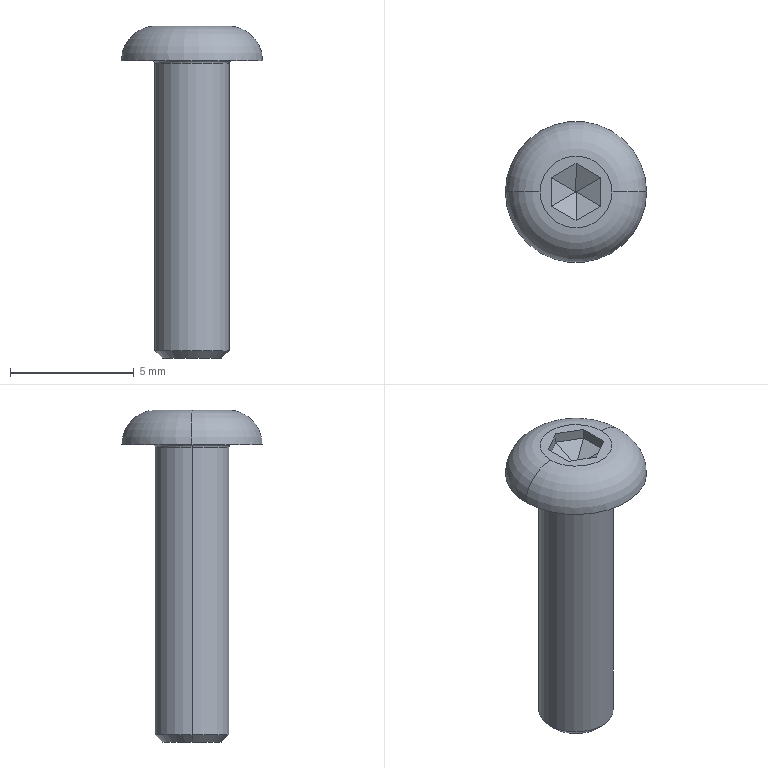Part | SolidWorks | features BaseBody 1 | 1 solid | 24 faces | box 5.7 x 5.7 x 13.4 mm | volume 111.333 mm3 | plane 16 | torus 4 | cone 2 | cylinder 2 | commonest cylinder face diameters 3 x2
STEP:
#1=CARTESIAN_POINT('',(-1.6,0.,0.));
#2=VERTEX_POINT('',#1);
#3=CARTESIAN_POINT('',(1.6,0.,0.));
#4=VERTEX_POINT('',#3);
#5=CARTESIAN_POINT('',(0.,0.,0.));
#6=DIRECTION('',(0.,0.,1.));
#7=DIRECTION('',(1.,0.,0.));
#8=AXIS2_PLACEMENT_3D('',#5,#6,#7);
#9=CIRCLE('',#8,1.6);
#10=EDGE_CURVE('',#2,#4,#9,.T.);
#11=ORIENTED_EDGE('',*,*,#10,.F.);
#12=CARTESIAN_POINT('',(-1.5,0.,-0.1));
#13=VERTEX_POINT('',#12);
#14=CARTESIAN_POINT('',(-1.6,0.,-0.1));
#15=DIRECTION('',(0.,1.,0.));
#16=DIRECTION('',(-1.,0.,0.));
#17=AXIS2_PLACEMENT_3D('',#14,#15,#16);
#18=CIRCLE('',#17,0.1);
#19=EDGE_CURVE('',#2,#13,#18,.T.);
#20=ORIENTED_EDGE('',*,*,#19,.T.);
#21=CARTESIAN_POINT('',(1.5,0.,-0.1));
#22=VERTEX_POINT('',#21);
#23=CARTESIAN_POINT('',(0.,0.,-0.1));
#24=DIRECTION('',(0.,0.,-1.));
#25=DIRECTION('',(1.,0.,0.));
#26=AXIS2_PLACEMENT_3D('',#23,#24,#25);
#27=CIRCLE('',#26,1.5);
#28=EDGE_CURVE('',#22,#13,#27,.T.);
#29=ORIENTED_EDGE('',*,*,#28,.F.);
#30=CARTESIAN_POINT('',(1.6,0.,-0.1));
#31=DIRECTION('',(0.,-1.,0.));
#32=DIRECTION('',(0.,0.,-1.));
#33=AXIS2_PLACEMENT_3D('',#30,#31,#32);
#34=CIRCLE('',#33,0.1);
#35=EDGE_CURVE('',#4,#22,#34,.T.);
#36=ORIENTED_EDGE('',*,*,#35,.F.);
#37=EDGE_LOOP('',(#11,#20,#29,#36));
#38=FACE_OUTER_BOUND('',#37,.T.);
#39=CARTESIAN_POINT('',(0.,0.,-0.1));
#40=DIRECTION('',(0.,0.,1.));
#41=DIRECTION('',(1.,0.,0.));
#42=AXIS2_PLACEMENT_3D('',#39,#40,#41);
#43=TOROIDAL_SURFACE('',#42,1.6,0.1);
#44=ADVANCED_FACE('',(#38),#43,.F.);
#45=CARTESIAN_POINT('',(-1.2,0.,-12.));
#46=VERTEX_POINT('',#45);
#47=CARTESIAN_POINT('',(1.2,0.,-12.));
#48=VERTEX_POINT('',#47);
#49=CARTESIAN_POINT('',(0.,0.,-12.));
#50=DIRECTION('',(0.,0.,-1.));
#51=DIRECTION('',(-1.,0.,0.));
#52=AXIS2_PLACEMENT_3D('',#49,#50,#51);
#53=CIRCLE('',#52,1.2);
#54=EDGE_CURVE('',#46,#48,#53,.T.);
#55=ORIENTED_EDGE('',*,*,#54,.F.);
#56=CARTESIAN_POINT('',(-1.5,0.,-11.7));
#57=VERTEX_POINT('',#56);
#58=CARTESIAN_POINT('',(-1.2,0.,-12.));
#59=DIRECTION('',(-0.7071,0.,0.7071));
#60=VECTOR('',#59,1000.);
#61=LINE('',#58,#60);
#62=EDGE_CURVE('',#46,#57,#61,.T.);
#63=ORIENTED_EDGE('',*,*,#62,.T.);
#64=CARTESIAN_POINT('',(1.5,0.,-11.7));
#65=VERTEX_POINT('',#64);
#66=CARTESIAN_POINT('',(0.,0.,-11.7));
#67=DIRECTION('',(0.,0.,1.));
#68=DIRECTION('',(-1.,0.,0.));
#69=AXIS2_PLACEMENT_3D('',#66,#67,#68);
#70=CIRCLE('',#69,1.5);
#71=EDGE_CURVE('',#65,#57,#70,.T.);
#72=ORIENTED_EDGE('',*,*,#71,.F.);
#73=CARTESIAN_POINT('',(1.2,0.,-12.));
#74=DIRECTION('',(0.7071,0.,0.7071));
#75=VECTOR('',#74,1000.);
#76=LINE('',#73,#75);
#77=EDGE_CURVE('',#48,#65,#76,.T.);
#78=ORIENTED_EDGE('',*,*,#77,.F.);
#79=EDGE_LOOP('',(#55,#63,#72,#78));
#80=FACE_OUTER_BOUND('',#79,.T.);
#81=CARTESIAN_POINT('',(0.,0.,-12.));
#82=DIRECTION('',(0.,0.,1.));
#83=DIRECTION('',(1.,0.,0.));
#84=AXIS2_PLACEMENT_3D('',#81,#82,#83);
#85=CONICAL_SURFACE('',#84,1.2,0.7854);
#86=ADVANCED_FACE('',(#80),#85,.T.);
#87=ORIENTED_EDGE('',*,*,#71,.T.);
#88=CARTESIAN_POINT('',(-1.5,0.,-12.));
#89=DIRECTION('',(0.,0.,1.));
#90=VECTOR('',#89,1000.);
#91=LINE('',#88,#90);
#92=EDGE_CURVE('',#57,#13,#91,.T.);
#93=ORIENTED_EDGE('',*,*,#92,.T.);
#94=CARTESIAN_POINT('',(0.,0.,-0.1));
#95=DIRECTION('',(0.,0.,-1.));
#96=DIRECTION('',(1.,0.,0.));
#97=AXIS2_PLACEMENT_3D('',#94,#95,#96);
#98=CIRCLE('',#97,1.5);
#99=EDGE_CURVE('',#13,#22,#98,.T.);
#100=ORIENTED_EDGE('',*,*,#99,.T.);
#101=CARTESIAN_POINT('',(1.5,0.,-12.));
#102=DIRECTION('',(0.,0.,1.));
#103=VECTOR('',#102,1000.);
#104=LINE('',#101,#103);
#105=EDGE_CURVE('',#65,#22,#104,.T.);
#106=ORIENTED_EDGE('',*,*,#105,.F.);
#107=EDGE_LOOP('',(#87,#93,#100,#106));
#108=FACE_OUTER_BOUND('',#107,.T.);
#109=CARTESIAN_POINT('',(0.,0.,-12.));
#110=DIRECTION('',(0.,0.,1.));
#111=DIRECTION('',(1.,0.,0.));
#112=AXIS2_PLACEMENT_3D('',#109,#110,#111);
#113=CYLINDRICAL_SURFACE('',#112,1.5);
#114=ADVANCED_FACE('',(#108),#113,.T.);
#115=CARTESIAN_POINT('',(2.85,0.,0.));
#116=VERTEX_POINT('',#115);
#117=CARTESIAN_POINT('',(-2.85,0.,0.));
#118=VERTEX_POINT('',#117);
#119=CARTESIAN_POINT('',(0.,0.,0.));
#120=DIRECTION('',(0.,0.,1.));
#121=DIRECTION('',(1.,0.,0.));
#122=AXIS2_PLACEMENT_3D('',#119,#120,#121);
#123=CIRCLE('',#122,2.85);
#124=EDGE_CURVE('',#116,#118,#123,.T.);
#125=ORIENTED_EDGE('',*,*,#124,.T.);
#126=CARTESIAN_POINT('',(-1.45,0.,1.4));
#127=VERTEX_POINT('',#126);
#128=CARTESIAN_POINT('',(-1.45,0.,0.));
#129=DIRECTION('',(0.,1.,0.));
#130=DIRECTION('',(-1.,0.,0.));
#131=AXIS2_PLACEMENT_3D('',#128,#129,#130);
#132=CIRCLE('',#131,1.4);
#133=EDGE_CURVE('',#118,#127,#132,.T.);
#134=ORIENTED_EDGE('',*,*,#133,.T.);
#135=CARTESIAN_POINT('',(1.45,0.,1.4));
#136=VERTEX_POINT('',#135);
#137=CARTESIAN_POINT('',(0.,0.,1.4));
#138=DIRECTION('',(0.,0.,1.));
#139=DIRECTION('',(1.,0.,0.));
#140=AXIS2_PLACEMENT_3D('',#137,#138,#139);
#141=CIRCLE('',#140,1.45);
#142=EDGE_CURVE('',#136,#127,#141,.T.);
#143=ORIENTED_EDGE('',*,*,#142,.F.);
#144=CARTESIAN_POINT('',(1.45,0.,0.));
#145=DIRECTION('',(0.,-1.,0.));
#146=DIRECTION('',(0.,0.,-1.));
#147=AXIS2_PLACEMENT_3D('',#144,#145,#146);
#148=CIRCLE('',#147,1.4);
#149=EDGE_CURVE('',#116,#136,#148,.T.);
#150=ORIENTED_EDGE('',*,*,#149,.F.);
#151=EDGE_LOOP('',(#125,#134,#143,#150));
#152=FACE_OUTER_BOUND('',#151,.T.);
#153=CARTESIAN_POINT('',(0.,0.,0.));
#154=DIRECTION('',(0.,0.,1.));
#155=DIRECTION('',(1.,0.,0.));
#156=AXIS2_PLACEMENT_3D('',#153,#154,#155);
#157=TOROIDAL_SURFACE('',#156,1.45,1.4);
#158=ADVANCED_FACE('',(#152),#157,.T.);
#159=CARTESIAN_POINT('',(-0.0017,-0.0009814,0.4));
#160=VERTEX_POINT('',#159);
#161=CARTESIAN_POINT('',(-1.,-0.5774,0.9764));
#162=VERTEX_POINT('',#161);
#163=CARTESIAN_POINT('',(-0.00136,-0.0007851,0.3998));
#164=DIRECTION('',(-0.7746,-0.4472,0.4472));
#165=VECTOR('',#164,1000.);
#166=LINE('',#163,#165);
#167=EDGE_CURVE('',#160,#162,#166,.T.);
#168=ORIENTED_EDGE('',*,*,#167,.T.);
#169=CARTESIAN_POINT('',(0.,-1.155,0.9764));
#170=VERTEX_POINT('',#169);
#171=CARTESIAN_POINT('',(-1.,-0.5774,0.9764));
#172=DIRECTION('',(-0.866,0.5,0.));
#173=VECTOR('',#172,1000.);
#174=LINE('',#171,#173);
#175=EDGE_CURVE('',#170,#162,#174,.T.);
#176=ORIENTED_EDGE('',*,*,#175,.F.);
#177=CARTESIAN_POINT('',(0.,-0.001963,0.4));
#178=VERTEX_POINT('',#177);
#179=CARTESIAN_POINT('',(0.,-0.00157,0.3998));
#180=DIRECTION('',(0.,0.8944,-0.4472));
#181=VECTOR('',#180,1000.);
#182=LINE('',#179,#181);
#183=EDGE_CURVE('',#170,#178,#182,.T.);
#184=ORIENTED_EDGE('',*,*,#183,.T.);
#185=CARTESIAN_POINT('',(-0.0008499,-0.001472,0.4));
#186=DIRECTION('',(0.866,-0.5,0.));
#187=VECTOR('',#186,1000.);
#188=LINE('',#185,#187);
#189=EDGE_CURVE('',#160,#178,#188,.T.);
#190=ORIENTED_EDGE('',*,*,#189,.F.);
#191=EDGE_LOOP('',(#168,#176,#184,#190));
#192=FACE_OUTER_BOUND('',#191,.T.);
#193=CARTESIAN_POINT('',(-0.0008499,-0.001472,0.4));
#194=DIRECTION('',(-0.25,-0.433,-0.866));
#195=DIRECTION('',(0.,-0.8944,0.4472));
#196=AXIS2_PLACEMENT_3D('',#193,#194,#195);
#197=PLANE('',#196);
#198=ADVANCED_FACE('',(#192),#197,.F.);
#199=CARTESIAN_POINT('',(1.,-0.5774,0.9764));
#200=VERTEX_POINT('',#199);
#201=CARTESIAN_POINT('',(0.0017,-0.0009814,0.4));
#202=VERTEX_POINT('',#201);
#203=CARTESIAN_POINT('',(0.00136,-0.0007851,0.3998));
#204=DIRECTION('',(-0.7746,0.4472,-0.4472));
#205=VECTOR('',#204,1000.);
#206=LINE('',#203,#205);
#207=EDGE_CURVE('',#200,#202,#206,.T.);
#208=ORIENTED_EDGE('',*,*,#207,.T.);
#209=CARTESIAN_POINT('',(0.0008499,-0.001472,0.4));
#210=DIRECTION('',(0.866,0.5,0.));
#211=VECTOR('',#210,1000.);
#212=LINE('',#209,#211);
#213=EDGE_CURVE('',#178,#202,#212,.T.);
#214=ORIENTED_EDGE('',*,*,#213,.F.);
#215=ORIENTED_EDGE('',*,*,#183,.F.);
#216=CARTESIAN_POINT('',(0.,-1.155,0.9764));
#217=DIRECTION('',(-0.866,-0.5,0.));
#218=VECTOR('',#217,1000.);
#219=LINE('',#216,#218);
#220=EDGE_CURVE('',#200,#170,#219,.T.);
#221=ORIENTED_EDGE('',*,*,#220,.F.);
#222=EDGE_LOOP('',(#208,#214,#215,#221));
#223=FACE_OUTER_BOUND('',#222,.T.);
#224=CARTESIAN_POINT('',(0.0008499,-0.001472,0.4));
#225=DIRECTION('',(0.25,-0.433,-0.866));
#226=DIRECTION('',(0.,-0.8944,0.4472));
#227=AXIS2_PLACEMENT_3D('',#224,#225,#226);
#228=PLANE('',#227);
#229=ADVANCED_FACE('',(#223),#228,.F.);
#230=CARTESIAN_POINT('',(-0.0017,0.0009814,0.4));
#231=VERTEX_POINT('',#230);
#232=CARTESIAN_POINT('',(-1.,0.5774,0.9764));
#233=VERTEX_POINT('',#232);
#234=CARTESIAN_POINT('',(-0.00136,0.0007851,0.3998));
#235=DIRECTION('',(-0.7746,0.4472,0.4472));
#236=VECTOR('',#235,1000.);
#237=LINE('',#234,#236);
#238=EDGE_CURVE('',#231,#233,#237,.T.);
#239=ORIENTED_EDGE('',*,*,#238,.T.);
#240=CARTESIAN_POINT('',(-1.,0.5774,0.9764));
#241=DIRECTION('',(0.,1.,0.));
#242=VECTOR('',#241,1000.);
#243=LINE('',#240,#242);
#244=EDGE_CURVE('',#162,#233,#243,.T.);
#245=ORIENTED_EDGE('',*,*,#244,.F.);
#246=ORIENTED_EDGE('',*,*,#167,.F.);
#247=CARTESIAN_POINT('',(-0.0017,0.,0.4));
#248=DIRECTION('',(0.,-1.,0.));
#249=VECTOR('',#248,1000.);
#250=LINE('',#247,#249);
#251=EDGE_CURVE('',#231,#160,#250,.T.);
#252=ORIENTED_EDGE('',*,*,#251,.F.);
#253=EDGE_LOOP('',(#239,#245,#246,#252));
#254=FACE_OUTER_BOUND('',#253,.T.);
#255=CARTESIAN_POINT('',(-0.0017,0.,0.4));
#256=DIRECTION('',(-0.5,0.,-0.866));
#257=DIRECTION('',(-0.866,0.,0.5));
#258=AXIS2_PLACEMENT_3D('',#255,#256,#257);
#259=PLANE('',#258);
#260=ADVANCED_FACE('',(#254),#259,.F.);
#261=CARTESIAN_POINT('',(1.,0.5774,0.9764));
#262=VERTEX_POINT('',#261);
#263=CARTESIAN_POINT('',(0.0017,0.0009814,0.4));
#264=VERTEX_POINT('',#263);
#265=CARTESIAN_POINT('',(0.00136,0.0007851,0.3998));
#266=DIRECTION('',(-0.7746,-0.4472,-0.4472));
#267=VECTOR('',#266,1000.);
#268=LINE('',#265,#267);
#269=EDGE_CURVE('',#262,#264,#268,.T.);
#270=ORIENTED_EDGE('',*,*,#269,.T.);
#271=CARTESIAN_POINT('',(0.0017,0.,0.4));
#272=DIRECTION('',(0.,1.,0.));
#273=VECTOR('',#272,1000.);
#274=LINE('',#271,#273);
#275=EDGE_CURVE('',#202,#264,#274,.T.);
#276=ORIENTED_EDGE('',*,*,#275,.F.);
#277=ORIENTED_EDGE('',*,*,#207,.F.);
#278=CARTESIAN_POINT('',(1.,-0.5774,0.9764));
#279=DIRECTION('',(0.,-1.,0.));
#280=VECTOR('',#279,1000.);
#281=LINE('',#278,#280);
#282=EDGE_CURVE('',#262,#200,#281,.T.);
#283=ORIENTED_EDGE('',*,*,#282,.F.);
#284=EDGE_LOOP('',(#270,#276,#277,#283));
#285=FACE_OUTER_BOUND('',#284,.T.);
#286=CARTESIAN_POINT('',(0.0017,0.,0.4));
#287=DIRECTION('',(0.5,0.,-0.866));
#288=DIRECTION('',(0.,-1.,0.));
#289=AXIS2_PLACEMENT_3D('',#286,#287,#288);
#290=PLANE('',#289);
#291=ADVANCED_FACE('',(#285),#290,.F.);
#292=CARTESIAN_POINT('',(0.,0.001963,0.4));
#293=VERTEX_POINT('',#292);
#294=CARTESIAN_POINT('',(0.,1.155,0.9764));
#295=VERTEX_POINT('',#294);
#296=CARTESIAN_POINT('',(0.,0.00157,0.3998));
#297=DIRECTION('',(0.,0.8944,0.4472));
#298=VECTOR('',#297,1000.);
#299=LINE('',#296,#298);
#300=EDGE_CURVE('',#293,#295,#299,.T.);
#301=ORIENTED_EDGE('',*,*,#300,.T.);
#302=CARTESIAN_POINT('',(0.,1.155,0.9764));
#303=DIRECTION('',(0.866,0.5,0.));
#304=VECTOR('',#303,1000.);
#305=LINE('',#302,#304);
#306=EDGE_CURVE('',#233,#295,#305,.T.);
#307=ORIENTED_EDGE('',*,*,#306,.F.);
#308=ORIENTED_EDGE('',*,*,#238,.F.);
#309=CARTESIAN_POINT('',(-0.0008499,0.001472,0.4));
#310=DIRECTION('',(-0.866,-0.5,0.));
#311=VECTOR('',#310,1000.);
#312=LINE('',#309,#311);
#313=EDGE_CURVE('',#293,#231,#312,.T.);
#314=ORIENTED_EDGE('',*,*,#313,.F.);
#315=EDGE_LOOP('',(#301,#307,#308,#314));
#316=FACE_OUTER_BOUND('',#315,.T.);
#317=CARTESIAN_POINT('',(-0.0008499,0.001472,0.4));
#318=DIRECTION('',(-0.25,0.433,-0.866));
#319=DIRECTION('',(-0.9608,0.,0.2774));
#320=AXIS2_PLACEMENT_3D('',#317,#318,#319);
#321=PLANE('',#320);
#322=ADVANCED_FACE('',(#316),#321,.F.);
#323=ORIENTED_EDGE('',*,*,#269,.F.);
#324=CARTESIAN_POINT('',(1.,0.5774,0.9764));
#325=DIRECTION('',(0.866,-0.5,0.));
#326=VECTOR('',#325,1000.);
#327=LINE('',#324,#326);
#328=EDGE_CURVE('',#295,#262,#327,.T.);
#329=ORIENTED_EDGE('',*,*,#328,.F.);
#330=ORIENTED_EDGE('',*,*,#300,.F.);
#331=CARTESIAN_POINT('',(0.0008499,0.001472,0.4));
#332=DIRECTION('',(-0.866,0.5,0.));
#333=VECTOR('',#332,1000.);
#334=LINE('',#331,#333);
#335=EDGE_CURVE('',#264,#293,#334,.T.);
#336=ORIENTED_EDGE('',*,*,#335,.F.);
#337=EDGE_LOOP('',(#323,#329,#330,#336));
#338=FACE_OUTER_BOUND('',#337,.T.);
#339=CARTESIAN_POINT('',(0.0008499,0.001472,0.4));
#340=DIRECTION('',(0.25,0.433,-0.866));
#341=DIRECTION('',(-0.9608,0.,-0.2774));
#342=AXIS2_PLACEMENT_3D('',#339,#340,#341);
#343=PLANE('',#342);
#344=ADVANCED_FACE('',(#338),#343,.F.);
#345=ORIENTED_EDGE('',*,*,#251,.T.);
#346=ORIENTED_EDGE('',*,*,#189,.T.);
#347=ORIENTED_EDGE('',*,*,#213,.T.);
#348=ORIENTED_EDGE('',*,*,#275,.T.);
#349=ORIENTED_EDGE('',*,*,#335,.T.);
#350=ORIENTED_EDGE('',*,*,#313,.T.);
#351=EDGE_LOOP('',(#345,#346,#347,#348,#349,#350));
#352=FACE_OUTER_BOUND('',#351,.T.);
#353=CARTESIAN_POINT('',(0.,0.,0.4));
#354=DIRECTION('',(0.,0.,1.));
#355=DIRECTION('',(1.,0.,0.));
#356=AXIS2_PLACEMENT_3D('',#353,#354,#355);
#357=PLANE('',#356);
#358=ADVANCED_FACE('',(#352),#357,.T.);
#359=CARTESIAN_POINT('',(0.,1.155,1.4));
#360=VERTEX_POINT('',#359);
#361=CARTESIAN_POINT('',(0.,1.155,0.4));
#362=DIRECTION('',(0.,0.,1.));
#363=VECTOR('',#362,1000.);
#364=LINE('',#361,#363);
#365=EDGE_CURVE('',#295,#360,#364,.T.);
#366=ORIENTED_EDGE('',*,*,#365,.F.);
#367=ORIENTED_EDGE('',*,*,#328,.T.);
#368=CARTESIAN_POINT('',(1.,0.5774,1.4));
#369=VERTEX_POINT('',#368);
#370=CARTESIAN_POINT('',(1.,0.5774,0.4));
#371=DIRECTION('',(0.,0.,1.));
#372=VECTOR('',#371,1000.);
#373=LINE('',#370,#372);
#374=EDGE_CURVE('',#262,#369,#373,.T.);
#375=ORIENTED_EDGE('',*,*,#374,.T.);
#376=CARTESIAN_POINT('',(1.,0.5774,1.4));
#377=DIRECTION('',(-0.866,0.5,0.));
#378=VECTOR('',#377,1000.);
#379=LINE('',#376,#378);
#380=EDGE_CURVE('',#369,#360,#379,.T.);
#381=ORIENTED_EDGE('',*,*,#380,.T.);
#382=EDGE_LOOP('',(#366,#367,#375,#381));
#383=FACE_OUTER_BOUND('',#382,.T.);
#384=CARTESIAN_POINT('',(1.,0.5774,0.4));
#385=DIRECTION('',(0.5,0.866,0.));
#386=DIRECTION('',(0.,0.,-1.));
#387=AXIS2_PLACEMENT_3D('',#384,#385,#386);
#388=PLANE('',#387);
#389=ADVANCED_FACE('',(#383),#388,.F.);
#390=CARTESIAN_POINT('',(-1.,0.5774,1.4));
#391=VERTEX_POINT('',#390);
#392=CARTESIAN_POINT('',(-1.,0.5774,0.4));
#393=DIRECTION('',(0.,0.,1.));
#394=VECTOR('',#393,1000.);
#395=LINE('',#392,#394);
#396=EDGE_CURVE('',#233,#391,#395,.T.);
#397=ORIENTED_EDGE('',*,*,#396,.F.);
#398=ORIENTED_EDGE('',*,*,#306,.T.);
#399=ORIENTED_EDGE('',*,*,#365,.T.);
#400=CARTESIAN_POINT('',(0.,1.155,1.4));
#401=DIRECTION('',(-0.866,-0.5,0.));
#402=VECTOR('',#401,1000.);
#403=LINE('',#400,#402);
#404=EDGE_CURVE('',#360,#391,#403,.T.);
#405=ORIENTED_EDGE('',*,*,#404,.T.);
#406=EDGE_LOOP('',(#397,#398,#399,#405));
#407=FACE_OUTER_BOUND('',#406,.T.);
#408=CARTESIAN_POINT('',(0.,1.155,0.4));
#409=DIRECTION('',(-0.5,0.866,0.));
#410=DIRECTION('',(0.,0.,1.));
#411=AXIS2_PLACEMENT_3D('',#408,#409,#410);
#412=PLANE('',#411);
#413=ADVANCED_FACE('',(#407),#412,.F.);
#414=CARTESIAN_POINT('',(-1.,-0.5774,1.4));
#415=VERTEX_POINT('',#414);
#416=CARTESIAN_POINT('',(-1.,-0.5774,0.4));
#417=DIRECTION('',(0.,0.,1.));
#418=VECTOR('',#417,1000.);
#419=LINE('',#416,#418);
#420=EDGE_CURVE('',#162,#415,#419,.T.);
#421=ORIENTED_EDGE('',*,*,#420,.F.);
#422=ORIENTED_EDGE('',*,*,#244,.T.);
#423=ORIENTED_EDGE('',*,*,#396,.T.);
#424=CARTESIAN_POINT('',(-1.,0.5774,1.4));
#425=DIRECTION('',(0.,-1.,0.));
#426=VECTOR('',#425,1000.);
#427=LINE('',#424,#426);
#428=EDGE_CURVE('',#391,#415,#427,.T.);
#429=ORIENTED_EDGE('',*,*,#428,.T.);
#430=EDGE_LOOP('',(#421,#422,#423,#429));
#431=FACE_OUTER_BOUND('',#430,.T.);
#432=CARTESIAN_POINT('',(-1.,0.5774,0.4));
#433=DIRECTION('',(-1.,0.,0.));
#434=DIRECTION('',(0.,0.,1.));
#435=AXIS2_PLACEMENT_3D('',#432,#433,#434);
#436=PLANE('',#435);
#437=ADVANCED_FACE('',(#431),#436,.F.);
#438=CARTESIAN_POINT('',(0.,-1.155,1.4));
#439=VERTEX_POINT('',#438);
#440=CARTESIAN_POINT('',(0.,-1.155,0.4));
#441=DIRECTION('',(0.,0.,1.));
#442=VECTOR('',#441,1000.);
#443=LINE('',#440,#442);
#444=EDGE_CURVE('',#170,#439,#443,.T.);
#445=ORIENTED_EDGE('',*,*,#444,.F.);
#446=ORIENTED_EDGE('',*,*,#175,.T.);
#447=ORIENTED_EDGE('',*,*,#420,.T.);
#448=CARTESIAN_POINT('',(-1.,-0.5774,1.4));
#449=DIRECTION('',(0.866,-0.5,0.));
#450=VECTOR('',#449,1000.);
#451=LINE('',#448,#450);
#452=EDGE_CURVE('',#415,#439,#451,.T.);
#453=ORIENTED_EDGE('',*,*,#452,.T.);
#454=EDGE_LOOP('',(#445,#446,#447,#453));
#455=FACE_OUTER_BOUND('',#454,.T.);
#456=CARTESIAN_POINT('',(-1.,-0.5774,0.4));
#457=DIRECTION('',(-0.5,-0.866,0.));
#458=DIRECTION('',(-0.866,0.5,0.));
#459=AXIS2_PLACEMENT_3D('',#456,#457,#458);
#460=PLANE('',#459);
#461=ADVANCED_FACE('',(#455),#460,.F.);
#462=CARTESIAN_POINT('',(1.,-0.5774,1.4));
#463=VERTEX_POINT('',#462);
#464=CARTESIAN_POINT('',(1.,-0.5774,0.4));
#465=DIRECTION('',(0.,0.,1.));
#466=VECTOR('',#465,1000.);
#467=LINE('',#464,#466);
#468=EDGE_CURVE('',#200,#463,#467,.T.);
#469=ORIENTED_EDGE('',*,*,#468,.F.);
#470=ORIENTED_EDGE('',*,*,#220,.T.);
#471=ORIENTED_EDGE('',*,*,#444,.T.);
#472=CARTESIAN_POINT('',(0.,-1.155,1.4));
#473=DIRECTION('',(0.866,0.5,0.));
#474=VECTOR('',#473,1000.);
#475=LINE('',#472,#474);
#476=EDGE_CURVE('',#439,#463,#475,.T.);
#477=ORIENTED_EDGE('',*,*,#476,.T.);
#478=EDGE_LOOP('',(#469,#470,#471,#477));
#479=FACE_OUTER_BOUND('',#478,.T.);
#480=CARTESIAN_POINT('',(0.,-1.155,0.4));
#481=DIRECTION('',(0.5,-0.866,0.));
#482=DIRECTION('',(0.,0.,-1.));
#483=AXIS2_PLACEMENT_3D('',#480,#481,#482);
#484=PLANE('',#483);
#485=ADVANCED_FACE('',(#479),#484,.F.);
#486=ORIENTED_EDGE('',*,*,#374,.F.);
#487=ORIENTED_EDGE('',*,*,#282,.T.);
#488=ORIENTED_EDGE('',*,*,#468,.T.);
#489=CARTESIAN_POINT('',(1.,-0.5774,1.4));
#490=DIRECTION('',(0.,1.,0.));
#491=VECTOR('',#490,1000.);
#492=LINE('',#489,#491);
#493=EDGE_CURVE('',#463,#369,#492,.T.);
#494=ORIENTED_EDGE('',*,*,#493,.T.);
#495=EDGE_LOOP('',(#486,#487,#488,#494));
#496=FACE_OUTER_BOUND('',#495,.T.);
#497=CARTESIAN_POINT('',(1.,-0.5774,0.4));
#498=DIRECTION('',(1.,0.,0.));
#499=DIRECTION('',(0.,1.,0.));
#500=AXIS2_PLACEMENT_3D('',#497,#498,#499);
#501=PLANE('',#500);
#502=ADVANCED_FACE('',(#496),#501,.F.);
#503=CARTESIAN_POINT('',(0.,0.,-12.));
#504=DIRECTION('',(0.,0.,-1.));
#505=DIRECTION('',(-1.,0.,0.));
#506=AXIS2_PLACEMENT_3D('',#503,#504,#505);
#507=CIRCLE('',#506,1.2);
#508=EDGE_CURVE('',#48,#46,#507,.T.);
#509=ORIENTED_EDGE('',*,*,#508,.T.);
#510=ORIENTED_EDGE('',*,*,#54,.T.);
#511=EDGE_LOOP('',(#509,#510));
#512=FACE_OUTER_BOUND('',#511,.T.);
#513=CARTESIAN_POINT('',(0.,0.,-12.));
#514=DIRECTION('',(0.,0.,-1.));
#515=DIRECTION('',(0.,-1.,0.));
#516=AXIS2_PLACEMENT_3D('',#513,#514,#515);
#517=PLANE('',#516);
#518=ADVANCED_FACE('',(#512),#517,.T.);
#519=ORIENTED_EDGE('',*,*,#493,.F.);
#520=ORIENTED_EDGE('',*,*,#476,.F.);
#521=ORIENTED_EDGE('',*,*,#452,.F.);
#522=ORIENTED_EDGE('',*,*,#428,.F.);
#523=ORIENTED_EDGE('',*,*,#404,.F.);
#524=ORIENTED_EDGE('',*,*,#380,.F.);
#525=EDGE_LOOP('',(#519,#520,#521,#522,#523,#524));
#526=FACE_BOUND('',#525,.T.);
#527=ORIENTED_EDGE('',*,*,#142,.T.);
#528=CARTESIAN_POINT('',(0.,0.,1.4));
#529=DIRECTION('',(0.,0.,1.));
#530=DIRECTION('',(1.,0.,0.));
#531=AXIS2_PLACEMENT_3D('',#528,#529,#530);
#532=CIRCLE('',#531,1.45);
#533=EDGE_CURVE('',#127,#136,#532,.T.);
#534=ORIENTED_EDGE('',*,*,#533,.T.);
#535=EDGE_LOOP('',(#527,#534));
#536=FACE_OUTER_BOUND('',#535,.T.);
#537=CARTESIAN_POINT('',(0.,0.,1.4));
#538=DIRECTION('',(0.,0.,1.));
#539=DIRECTION('',(1.,0.,0.));
#540=AXIS2_PLACEMENT_3D('',#537,#538,#539);
#541=PLANE('',#540);
#542=ADVANCED_FACE('',(#526,#536),#541,.T.);
#543=CARTESIAN_POINT('',(0.,0.,0.));
#544=DIRECTION('',(0.,0.,1.));
#545=DIRECTION('',(1.,0.,0.));
#546=AXIS2_PLACEMENT_3D('',#543,#544,#545);
#547=CIRCLE('',#546,1.6);
#548=EDGE_CURVE('',#4,#2,#547,.T.);
#549=ORIENTED_EDGE('',*,*,#548,.T.);
#550=ORIENTED_EDGE('',*,*,#10,.T.);
#551=EDGE_LOOP('',(#549,#550));
#552=FACE_BOUND('',#551,.T.);
#553=ORIENTED_EDGE('',*,*,#124,.F.);
#554=CARTESIAN_POINT('',(0.,0.,0.));
#555=DIRECTION('',(0.,0.,1.));
#556=DIRECTION('',(1.,0.,0.));
#557=AXIS2_PLACEMENT_3D('',#554,#555,#556);
#558=CIRCLE('',#557,2.85);
#559=EDGE_CURVE('',#118,#116,#558,.T.);
#560=ORIENTED_EDGE('',*,*,#559,.F.);
#561=EDGE_LOOP('',(#553,#560));
#562=FACE_OUTER_BOUND('',#561,.T.);
#563=CARTESIAN_POINT('',(0.,0.,0.));
#564=DIRECTION('',(0.,0.,1.));
#565=DIRECTION('',(1.,0.,0.));
#566=AXIS2_PLACEMENT_3D('',#563,#564,#565);
#567=PLANE('',#566);
#568=ADVANCED_FACE('',(#552,#562),#567,.F.);
#569=ORIENTED_EDGE('',*,*,#133,.F.);
#570=ORIENTED_EDGE('',*,*,#559,.T.);
#571=ORIENTED_EDGE('',*,*,#149,.T.);
#572=ORIENTED_EDGE('',*,*,#533,.F.);
#573=EDGE_LOOP('',(#569,#570,#571,#572));
#574=FACE_OUTER_BOUND('',#573,.T.);
#575=CARTESIAN_POINT('',(0.,0.,0.));
#576=DIRECTION('',(0.,0.,1.));
#577=DIRECTION('',(1.,0.,0.));
#578=AXIS2_PLACEMENT_3D('',#575,#576,#577);
#579=TOROIDAL_SURFACE('',#578,1.45,1.4);
#580=ADVANCED_FACE('',(#574),#579,.T.);
#581=ORIENTED_EDGE('',*,*,#92,.F.);
#582=CARTESIAN_POINT('',(0.,0.,-11.7));
#583=DIRECTION('',(0.,0.,1.));
#584=DIRECTION('',(-1.,0.,0.));
#585=AXIS2_PLACEMENT_3D('',#582,#583,#584);
#586=CIRCLE('',#585,1.5);
#587=EDGE_CURVE('',#57,#65,#586,.T.);
#588=ORIENTED_EDGE('',*,*,#587,.T.);
#589=ORIENTED_EDGE('',*,*,#105,.T.);
#590=ORIENTED_EDGE('',*,*,#28,.T.);
#591=EDGE_LOOP('',(#581,#588,#589,#590));
#592=FACE_OUTER_BOUND('',#591,.T.);
#593=CARTESIAN_POINT('',(0.,0.,-12.));
#594=DIRECTION('',(0.,0.,1.));
#595=DIRECTION('',(1.,0.,0.));
#596=AXIS2_PLACEMENT_3D('',#593,#594,#595);
#597=CYLINDRICAL_SURFACE('',#596,1.5);
#598=ADVANCED_FACE('',(#592),#597,.T.);
#599=ORIENTED_EDGE('',*,*,#62,.F.);
#600=ORIENTED_EDGE('',*,*,#508,.F.);
#601=ORIENTED_EDGE('',*,*,#77,.T.);
#602=ORIENTED_EDGE('',*,*,#587,.F.);
#603=EDGE_LOOP('',(#599,#600,#601,#602));
#604=FACE_OUTER_BOUND('',#603,.T.);
#605=CARTESIAN_POINT('',(0.,0.,-12.));
#606=DIRECTION('',(0.,0.,1.));
#607=DIRECTION('',(1.,0.,0.));
#608=AXIS2_PLACEMENT_3D('',#605,#606,#607);
#609=CONICAL_SURFACE('',#608,1.2,0.7854);
#610=ADVANCED_FACE('',(#604),#609,.T.);
#611=ORIENTED_EDGE('',*,*,#19,.F.);
#612=ORIENTED_EDGE('',*,*,#548,.F.);
#613=ORIENTED_EDGE('',*,*,#35,.T.);
#614=ORIENTED_EDGE('',*,*,#99,.F.);
#615=EDGE_LOOP('',(#611,#612,#613,#614));
#616=FACE_OUTER_BOUND('',#615,.T.);
#617=CARTESIAN_POINT('',(0.,0.,-0.1));
#618=DIRECTION('',(0.,0.,1.));
#619=DIRECTION('',(1.,0.,0.));
#620=AXIS2_PLACEMENT_3D('',#617,#618,#619);
#621=TOROIDAL_SURFACE('',#620,1.6,0.1);
#622=ADVANCED_FACE('',(#616),#621,.F.);
#623=CLOSED_SHELL('',(#44,#86,#114,#158,#198,#229,#260,#291,#322,#344,#358,#389,#413,#437,#461,#485,#502,#518,#542,#568,#580,#598,#610,#622));
#624=MANIFOLD_SOLID_BREP('',#623);
#625=CARTESIAN_POINT('',(0.,0.,0.));
#626=DIRECTION('',(0.,0.,1.));
#627=DIRECTION('',(1.,0.,0.));
#628=AXIS2_PLACEMENT_3D('',#625,#626,#627);
#629=(LENGTH_UNIT()NAMED_UNIT(*)SI_UNIT(.MILLI.,.METRE.));
#630=UNCERTAINTY_MEASURE_WITH_UNIT(LENGTH_MEASURE(0.00001),#629,'','');
#631=(NAMED_UNIT(*)PLANE_ANGLE_UNIT()SI_UNIT($,.RADIAN.));
#632=(NAMED_UNIT(*)SI_UNIT($,.STERADIAN.)SOLID_ANGLE_UNIT());
#633=(GEOMETRIC_REPRESENTATION_CONTEXT(3)GLOBAL_UNCERTAINTY_ASSIGNED_CONTEXT((#630))GLOBAL_UNIT_ASSIGNED_CONTEXT((#629,#631,#632))REPRESENTATION_CONTEXT('',''));
#634=ADVANCED_BREP_SHAPE_REPRESENTATION('',(#624,#628),#633);